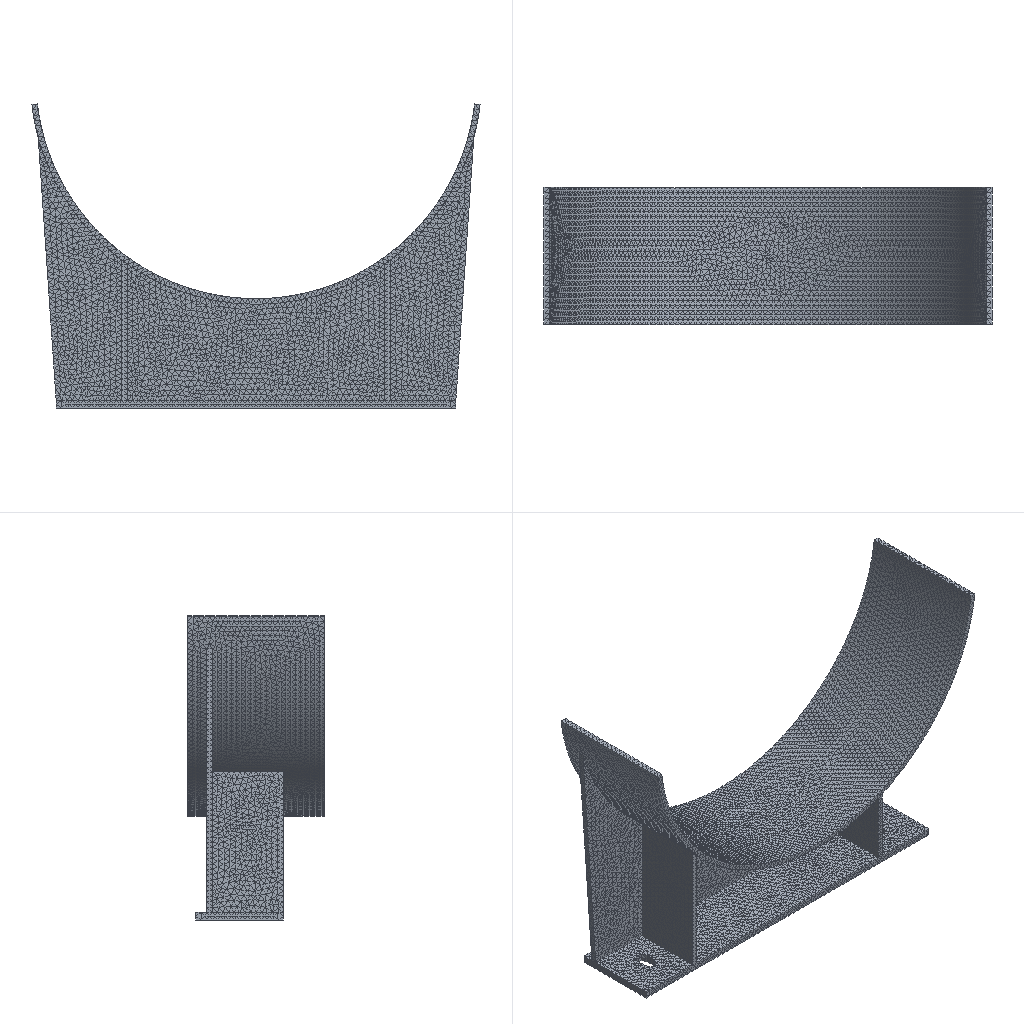Simulation study | ansys workbench
Set-up summary:
category,name,step,type,value,unit,region
solver,ansys_workbench
units,mm-N-s-tonne (MPa),,stated,"/units,MPA"
analysis,LS1,,static
load_step,LS1,LS1,static,nsubst=1; time=1
mesh,nodes,,,97537
mesh,elements,,,56993
element_type,SOLID187,,,50409
element_type,SURF154,,,6584
material,Q235B,,E,206000,tonne s^-2 mm^-1
material,Q235B,,nu,0.3
material,Q235B,,density,7.85e-09,tonne mm^-3
load,Define Force Using Surface Effect Elements,LS1,surface-effect pres face 3,-0.08104,,SURF154 #2
bc,Fixed Supports,model,fixed,[dofs=ALL],,_FIXEDSU
named_set,_FIXEDSU,,node,5117
Ansys APDL input file, long lists of numbers shortened:
/batch
/config,noeldb,1     ! force off writing results to database
*get,_wallstrt,active,,time,wall
! ANSYS input file written by Workbench version 2022 R2
! File used for geometry attach:
/title,wbnew--____ (A5)
! ****** Begin Custom Load Command Snippet ******
/COM, ACT Extensions:
/COM,     LSDYNA, 2022.2
/COM,/COM,     ANSYSMotion, 2022.2
/COM,
! ****** End   Custom Load Command Snippet ******
*DIM,_wb_ProjectScratch_dir,string,248
_wb_ProjectScratch_dir(1) = ''
*DIM,_wb_SolverFiles_dir,string,248
_wb_SolverFiles_dir(1) = ''
*DIM,_wb_userfiles_dir,string,248
_wb_userfiles_dir(1) = ''
/com,--- Data in consistent NMM units. See Solving Units in the help system for more information.
/units,MPA
/nopr
/wb,file,start              !  signify a WB generated input file
/prep7
! Turn off shape checking because checks already performed inside WB mesher.
! See help system for more information.
SHPP,OFF,,NOWARN
/nolist
etcon,set             ! allow ANSYS to choose best KEYOP's for 180x elements, resets any applicable keyopt to MAPDL defaults
/com,*********** Nodes for the whole assembly ***********
nblock,3,,107290
(1i9,3e20.9e3)
        1     3.690000000E+02    -1.108524441E+02     2.000199010E+02
! (97536 more lines like these left out)
-1
/wb,elem,start            !  set before creation of elements
/com,*********** Elements for Body 1 "__-FreeParts|NONE" ***********
et,1,187
eblock,19,solid,,50409
(19i9)
        1        1        1        1        0        0        0        0       10        0        1    14587    16005    16088    16006    94254    97528    94256    94255
! (100817 more lines like these left out)
-1
/wb,elem,end               !  done creating elements
/com,*********** Send User Defined Coordinate System(s) ***********
csys,0
toffst,273.15,  ! Temperature offset from absolute zero
/com,*********** Set Reference Temperature ***********
tref,22.
/wb,mat,start              !  starting to send materials
/com,*********** Send Materials ***********
MP,DENS,1,7.85e-09,	! tonne mm^-3
MP,EX,1,206000,	! tonne s^-2 mm^-1
MP,NUXY,1,0.3,
/wb,mat,end                !  done sending materials
!************************* Model Summary ********************
!__-FreeParts|NONE,	Q235B,	matid,	1
!************************* End Model Summary ********************
! get the diagonal of the bounding box. Needed later for other things
*get,_xmin,node,,mnloc,x
*get,_ymin,node,,mnloc,y
*get,_zmin,node,,mnloc,z
*get,_xmax,node,,mxloc,x
*get,_ymax,node,,mxloc,y
*get,_zmax,node,,mxloc,z
_ASMDIAG=(_xmax-_xmin)*(_xmax-_xmin)+(_ymax-_ymin)*(_ymax-_ymin)+(_zmax-_zmin)*(_zmax-_zmin)
_ASMDIAG=SQRT(_ASMDIAG)
/wb,contact,start          !  starting to send contact
/wb,contact,end            !  done creating contacts
/golist
/wb,load,start             !  starting to send loads
/com,*********** Fixed Supports ***********
CMBLOCK,_FIXEDSU,NODE,     5117
(8i10)
       928       929       930       931       932       933       934       935
! (639 more lines like these left out)
cmsel,s,_FIXEDSU
d,all,all
nsel,all
/com,*********** Define Force Using Surface Effect Elements ***********
local,12,0,0.,0.,0.,0.,0.,0.
csys,0
et,2,154
eblock,10,,,6584
(15i9)
    80310        2        2        2       12      115      116     4891     4891    16774    16784     4891    16779
! (6583 more lines like these left out)
-1
esel,s,type,,2
keyop,2,2,1                ! Apply load in local coordinate system
keyop,2,7,1                ! Use original area so load is constant in large deformation
esel,all
/gst,on,on
fini
*get,_numnode,node,0,count
*get,_numelem,elem,0,count
*get, _MAXELEMNUM, elem, 0, NUM, MAX
*get, _MAXNODENUM, node, 0, NUM, MAX
*get, _MAXELEMTYPE, etyp, 0, NUM, MAX
*get, _MAXREALCONST, rcon, 0, NUM, MAX
/go
/wb,load,end               !  done creating loads
/com,--- Number of total nodes = %_numnode%
/com,--- Number of contact elements = 6584
/com,--- Number of spring elements = 0
/com,--- Number of bearing elements = 0
/com,--- Number of solid elements = 50409
/com,--- Number of condensed parts = 0
/com,--- Number of total elements = %_numelem%
*get,_wallbsol,active,,time,wall
/com,****************************************************************************
/com,*************************    SOLUTION       ********************************
/com,****************************************************************************
/solu
antype,0                   ! static analysis
_thickRatio=  0     ! Ratio of thick parts in the model
eqsl,sparse,,,,,1
cntr,print,1               ! print out contact info and also make no initial contact an error
dmpoption,emat,no             ! Don't combine emat file for DANSYS
dmpoption,esav,no             ! Don't combine esav file for DANSYS
nldiag,cont,iter           ! print out contact info each equilibrium iteration
rescontrol,,none                 ! Do not keep any restart files
/com,****************************************************
/com,******************* SOLVE FOR LS 1 OF 1 ****************
esel,s,type,,2
nsle
sfe,all,1,pres,1,0.
sfe,all,2,pres,1,0.
sfe,all,3,pres,1,-8.10437974016225e-002
nsel,all
esel,all
/nopr
/gopr
nsub,1,1,1
time,1.
outres,erase
outres,all,none
outres,nsol,all,
outres,rsol,all
outres,eangl,all
outres,etmp,all
outres,veng,all
outres,strs,all,
outres,epel,all,
outres,eppl,all,
outres,cont,all,
! *********** WB SOLVE COMMAND ***********
! check interactive state
*get,ANSINTER_,active,,int
*if,ANSINTER_,ne,0,then
/eof
*endif
solve
/com *************** Write FE CONNECTORS *********
CEWRITE,file,ce,,INTE
/com,****************************************************
/com,*************** FINISHED SOLVE FOR LS 1 *************
*get,_wallasol,active,,time,wall
/nopr
*get,_numnode,node,0,count
*get,_numelem,elem,0,count
*get, _MAXELEMNUM, elem, 0, NUM, MAX
*get, _MAXNODENUM, node, 0, NUM, MAX,,,INTERNAL
*get, _MAXELEMTYPE, etyp, 0, NUM, MAX
*get, _MAXREALCONST, rcon, 0, NUM, MAX
*get,_NSOLTHREADS,active,0,ntfs
*get,_NSOLPROCESSES,active,0,npfs
/gopr
/post1
xmlo,ENCODING,ISO-8859-1
xmlo,parm
/xml,parm,xml
fini
/gopr
*get,_walldone,active,,time,wall
_preptime=(_wallbsol-_wallstrt)*3600
_solvtime=(_wallasol-_wallbsol)*3600
_posttime=(_walldone-_wallasol)*3600
_totaltim=(_walldone-_wallstrt)*3600
*get,_dlbratio,active,0,solu,dlbr
*get,_combtime,active,0,solu,comb
*get,_ssmode,active,0,solu,ssmm
*get,_ndofs,active,0,solu,ndof
*get,_sol_end_time,active,0,set,time
*if,_sol_end_time,eq,1.,then
/fclean				!clean distributed files
*endif
/com,--- Total number of nodes = %_numnode%
/com,--- Total number of elements = %_numelem%
/com,--- Element load balance ratio = %_dlbratio%
/com,--- Time to combine distributed files = %_combtime%
/com,--- Sparse memory mode = %_ssmode%
/com,--- Number of DOF = %_ndofs%
/wb,file,end               ! done with WB generated input
Results summary:
result,analyses[0].index,,,1
result,analyses[0].system,,,SYS
result,analyses[0].deck,,,deck.dat
result,analyses[0].solve_status,,,completed
result,analyses[0].analysis_type,,,static
result,analyses[0].physics,,,mechanical
result,analyses[0].unit_system,,,"NMM: mm, ton, N, s, mV, mA, degC"
result,analyses[0].n_sets,,,1
result,analyses[0].load_steps[0].set,set=1,,1
result,analyses[0].load_steps[0].time_or_freq,set=1,,1
result,analyses[0].load_steps[0].max_displacement_magnitude,set=1,,1.104
result,analyses[0].load_steps[0].max_von_mises_nodal,set=1,,89.693
result,analyses[0].load_steps[0].reaction_force_sum_xyz[1],set=1,,4.22451e-07
result,analyses[0].load_steps[0].reaction_force_sum_xyz[2],set=1,,2.26101e-07
result,analyses[0].load_steps[0].reaction_force_sum_xyz[3],set=1,,23700